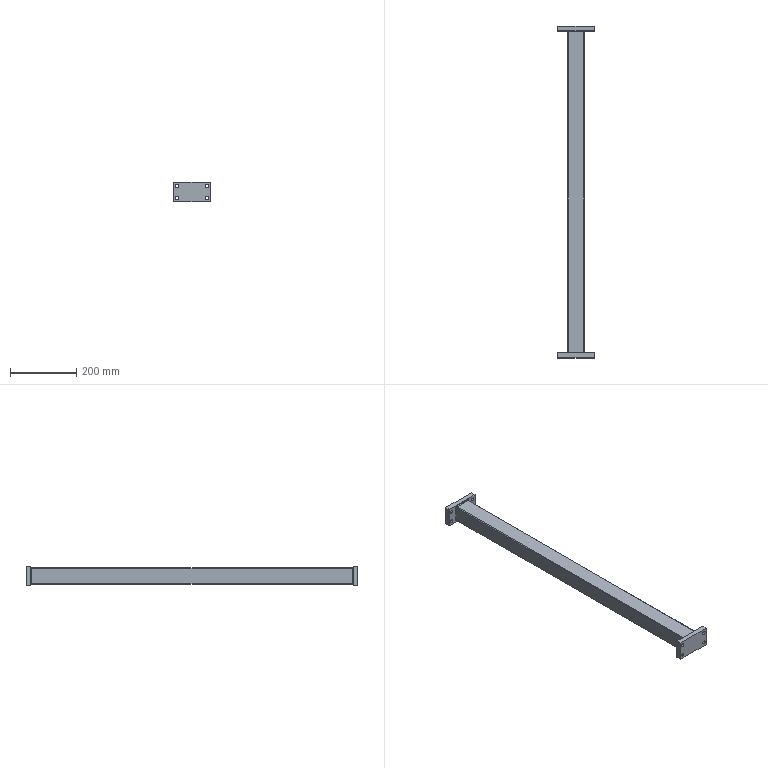Part | STEP file | Reinforcing rod XG | 1 solid | 58 faces | box 110 x 1000 x 60 mm | volume 1058206 mm3 | cylinder 28 | plane 22 | torus 8 | commonest cylinder face diameters 10.2 x16 4 x12